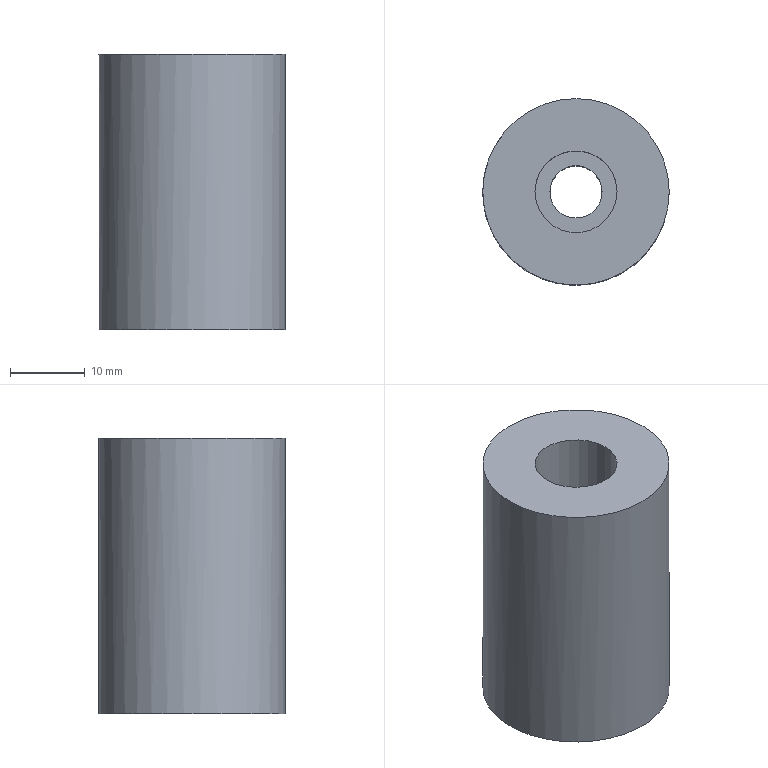Part | NX | features DIE-13 2 | 1 solid | 6 faces | box 25 x 25 x 36.9 mm | volume 16188 mm3 | cylinder 3 | plane 3 | commonest cylinder face diameters 7.007 x1 11 x1 25 x1
STEP:
#1=CARTESIAN_POINT('',(3653.586,-743.422,860.616));
#2=VERTEX_POINT('',#1);
#3=CARTESIAN_POINT('',(3666.086,-743.422,860.616));
#4=DIRECTION('',(0.,0.,1.));
#5=DIRECTION('',(-1.,0.,0.));
#6=AXIS2_PLACEMENT_3D('',#3,#4,#5);
#7=CIRCLE('',#6,12.5);
#8=EDGE_CURVE('',#2,#2,#7,.T.);
#9=ORIENTED_EDGE('',*,*,#8,.F.);
#10=EDGE_LOOP('',(#9));
#11=FACE_BOUND('',#10,.T.);
#12=CARTESIAN_POINT('',(3678.586,-743.422,823.716));
#13=VERTEX_POINT('',#12);
#14=CARTESIAN_POINT('',(3666.086,-743.422,823.716));
#15=DIRECTION('',(0.,0.,-1.));
#16=DIRECTION('',(1.,0.,0.));
#17=AXIS2_PLACEMENT_3D('',#14,#15,#16);
#18=CIRCLE('',#17,12.5);
#19=EDGE_CURVE('',#13,#13,#18,.T.);
#20=ORIENTED_EDGE('',*,*,#19,.F.);
#21=EDGE_LOOP('',(#20));
#22=FACE_BOUND('',#21,.T.);
#23=CARTESIAN_POINT('',(3666.086,-743.422,823.716));
#24=DIRECTION('',(0.,0.,1.));
#25=DIRECTION('',(1.,0.,0.));
#26=AXIS2_PLACEMENT_3D('',#23,#24,#25);
#27=CYLINDRICAL_SURFACE('',#26,12.5);
#28=ADVANCED_FACE('',(#11,#22),#27,.T.);
#29=CARTESIAN_POINT('',(3660.586,-743.422,860.616));
#30=VERTEX_POINT('',#29);
#31=CARTESIAN_POINT('',(3666.086,-743.422,860.616));
#32=DIRECTION('',(0.,0.,1.));
#33=DIRECTION('',(-1.,0.,0.));
#34=AXIS2_PLACEMENT_3D('',#31,#32,#33);
#35=CIRCLE('',#34,5.5);
#36=EDGE_CURVE('',#30,#30,#35,.T.);
#37=ORIENTED_EDGE('',*,*,#36,.T.);
#38=EDGE_LOOP('',(#37));
#39=FACE_BOUND('',#38,.T.);
#40=CARTESIAN_POINT('',(3660.586,-743.422,851.716));
#41=VERTEX_POINT('',#40);
#42=CARTESIAN_POINT('',(3666.086,-743.422,851.716));
#43=DIRECTION('',(0.,0.,1.));
#44=DIRECTION('',(-1.,0.,0.));
#45=AXIS2_PLACEMENT_3D('',#42,#43,#44);
#46=CIRCLE('',#45,5.5);
#47=EDGE_CURVE('',#41,#41,#46,.F.);
#48=ORIENTED_EDGE('',*,*,#47,.T.);
#49=EDGE_LOOP('',(#48));
#50=FACE_BOUND('',#49,.T.);
#51=CARTESIAN_POINT('',(3666.086,-743.422,859.966));
#52=DIRECTION('',(0.,0.,-1.));
#53=DIRECTION('',(1.,0.,0.));
#54=AXIS2_PLACEMENT_3D('',#51,#52,#53);
#55=CYLINDRICAL_SURFACE('',#54,5.5);
#56=ADVANCED_FACE('',(#39,#50),#55,.F.);
#57=ORIENTED_EDGE('',*,*,#36,.F.);
#58=EDGE_LOOP('',(#57));
#59=FACE_BOUND('',#58,.T.);
#60=ORIENTED_EDGE('',*,*,#8,.T.);
#61=EDGE_LOOP('',(#60));
#62=FACE_BOUND('',#61,.T.);
#63=CARTESIAN_POINT('',(2239.151,-594.707,860.616));
#64=DIRECTION('',(0.,0.,-1.));
#65=DIRECTION('',(1.,0.,0.));
#66=AXIS2_PLACEMENT_3D('',#63,#64,#65);
#67=PLANE('',#66);
#68=ADVANCED_FACE('',(#59,#62),#67,.F.);
#69=CARTESIAN_POINT('',(3662.582,-743.422,851.716));
#70=VERTEX_POINT('',#69);
#71=CARTESIAN_POINT('',(3666.086,-743.422,851.716));
#72=DIRECTION('',(0.,0.,1.));
#73=DIRECTION('',(-1.,0.,0.));
#74=AXIS2_PLACEMENT_3D('',#71,#72,#73);
#75=CIRCLE('',#74,3.503);
#76=EDGE_CURVE('',#70,#70,#75,.T.);
#77=ORIENTED_EDGE('',*,*,#76,.F.);
#78=EDGE_LOOP('',(#77));
#79=FACE_BOUND('',#78,.T.);
#80=ORIENTED_EDGE('',*,*,#47,.F.);
#81=EDGE_LOOP('',(#80));
#82=FACE_BOUND('',#81,.T.);
#83=CARTESIAN_POINT('',(3666.086,-743.422,851.716));
#84=DIRECTION('',(0.,0.,-1.));
#85=DIRECTION('',(-1.,0.,0.));
#86=AXIS2_PLACEMENT_3D('',#83,#84,#85);
#87=PLANE('',#86);
#88=ADVANCED_FACE('',(#79,#82),#87,.F.);
#89=ORIENTED_EDGE('',*,*,#19,.T.);
#90=EDGE_LOOP('',(#89));
#91=FACE_BOUND('',#90,.T.);
#92=CARTESIAN_POINT('',(3669.589,-743.422,823.716));
#93=VERTEX_POINT('',#92);
#94=CARTESIAN_POINT('',(3666.086,-743.422,823.716));
#95=DIRECTION('',(0.,0.,-1.));
#96=DIRECTION('',(1.,0.,0.));
#97=AXIS2_PLACEMENT_3D('',#94,#95,#96);
#98=CIRCLE('',#97,3.503);
#99=EDGE_CURVE('',#93,#93,#98,.F.);
#100=ORIENTED_EDGE('',*,*,#99,.T.);
#101=EDGE_LOOP('',(#100));
#102=FACE_BOUND('',#101,.T.);
#103=CARTESIAN_POINT('',(3541.577,-625.722,823.716));
#104=DIRECTION('',(0.,0.,1.));
#105=DIRECTION('',(1.,0.,0.));
#106=AXIS2_PLACEMENT_3D('',#103,#104,#105);
#107=PLANE('',#106);
#108=ADVANCED_FACE('',(#91,#102),#107,.F.);
#109=ORIENTED_EDGE('',*,*,#76,.T.);
#110=EDGE_LOOP('',(#109));
#111=FACE_BOUND('',#110,.T.);
#112=ORIENTED_EDGE('',*,*,#99,.F.);
#113=EDGE_LOOP('',(#112));
#114=FACE_BOUND('',#113,.T.);
#115=CARTESIAN_POINT('',(3666.086,-743.422,859.966));
#116=DIRECTION('',(0.,0.,-1.));
#117=DIRECTION('',(1.,0.,0.));
#118=AXIS2_PLACEMENT_3D('',#115,#116,#117);
#119=CYLINDRICAL_SURFACE('',#118,3.503);
#120=ADVANCED_FACE('',(#111,#114),#119,.F.);
#121=CLOSED_SHELL('',(#28,#56,#68,#88,#108,#120));
#122=MANIFOLD_SOLID_BREP('',#121);
#123=(LENGTH_UNIT()NAMED_UNIT(*)SI_UNIT(.MILLI.,.METRE.));
#124=UNCERTAINTY_MEASURE_WITH_UNIT(LENGTH_MEASURE(0.00001),#123,'','');
#125=(NAMED_UNIT(*)PLANE_ANGLE_UNIT()SI_UNIT($,.RADIAN.));
#126=(NAMED_UNIT(*)SI_UNIT($,.STERADIAN.)SOLID_ANGLE_UNIT());
#127=(GEOMETRIC_REPRESENTATION_CONTEXT(3)GLOBAL_UNCERTAINTY_ASSIGNED_CONTEXT((#124))GLOBAL_UNIT_ASSIGNED_CONTEXT((#123,#125,#126))REPRESENTATION_CONTEXT('',''));
#128=ADVANCED_BREP_SHAPE_REPRESENTATION('',(#122),#127);